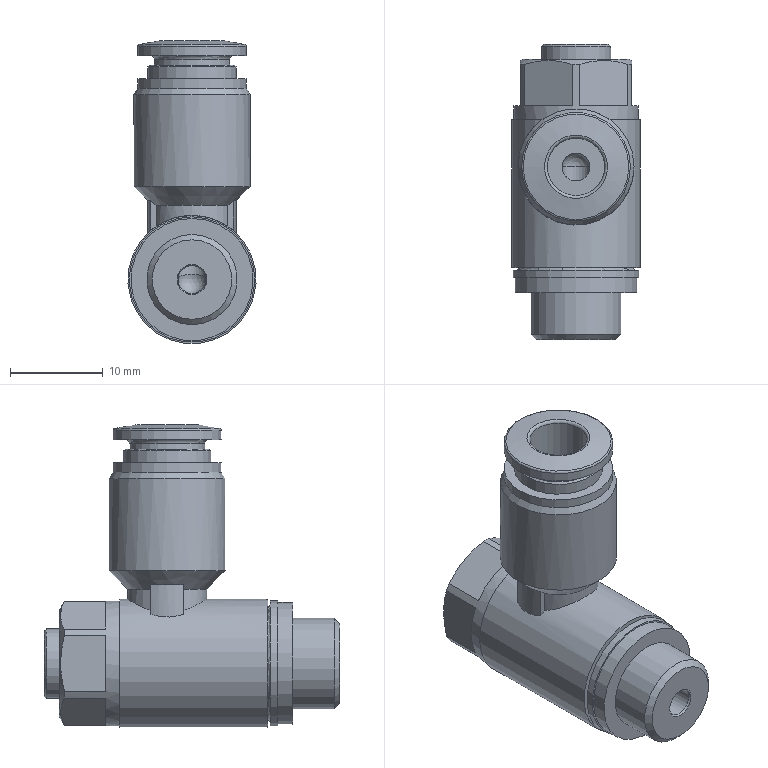Part | NX | features BREP 1 | 1 solid | 69 faces | box 13.8 x 31.75 x 32.6 mm | volume 5271 mm3 | plane 35 | cylinder 19 | cone 10 | torus 4 | sphere 1 | commonest cylinder face diameters 9.5 x3 3 x2 8.5 x2 11.7 x2 6.2 x1 6.3 x1